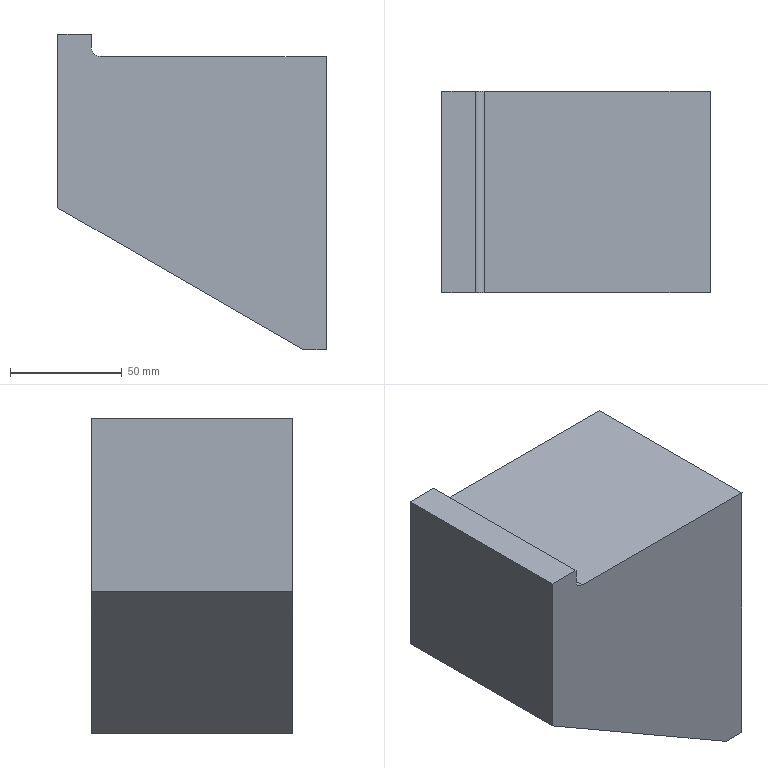Part | NX | features solid 2 | 1 solid | 10 faces | box 120 x 90 x 141.188 mm | volume 1116272 mm3 | plane 8 | spline 1 | cylinder 1 | commonest cylinder face diameters 8 x1
STEP:
#1=CARTESIAN_POINT('',(-871.,-430.,-90.));
#2=VERTEX_POINT('',#1);
#3=CARTESIAN_POINT('',(-770.,-430.,-90.));
#4=VERTEX_POINT('',#3);
#5=CARTESIAN_POINT('',(-871.,-430.,-90.));
#6=CARTESIAN_POINT('',(-837.333,-430.,-90.));
#7=CARTESIAN_POINT('',(-803.667,-430.,-90.));
#8=CARTESIAN_POINT('',(-770.,-430.,-90.));
#9=B_SPLINE_CURVE_WITH_KNOTS('',3,(#5,#6,#7,#8),.UNSPECIFIED.,.F.,.F.,(4,4),(0.1583,1.),.UNSPECIFIED.);
#10=EDGE_CURVE('',#2,#4,#9,.T.);
#11=ORIENTED_EDGE('',*,*,#10,.T.);
#12=CARTESIAN_POINT('',(-770.,-340.,-90.));
#13=VERTEX_POINT('',#12);
#14=CARTESIAN_POINT('',(-770.,-430.,-90.));
#15=CARTESIAN_POINT('',(-770.,-400.,-90.));
#16=CARTESIAN_POINT('',(-770.,-370.,-90.));
#17=CARTESIAN_POINT('',(-770.,-340.,-90.));
#18=B_SPLINE_CURVE_WITH_KNOTS('',3,(#14,#15,#16,#17),.UNSPECIFIED.,.F.,.F.,(4,4),(0.,1.),.UNSPECIFIED.);
#19=EDGE_CURVE('',#4,#13,#18,.T.);
#20=ORIENTED_EDGE('',*,*,#19,.T.);
#21=CARTESIAN_POINT('',(-871.,-340.,-90.));
#22=VERTEX_POINT('',#21);
#23=CARTESIAN_POINT('',(-770.,-340.,-90.));
#24=CARTESIAN_POINT('',(-803.667,-340.,-90.));
#25=CARTESIAN_POINT('',(-837.333,-340.,-90.));
#26=CARTESIAN_POINT('',(-871.,-340.,-90.));
#27=B_SPLINE_CURVE_WITH_KNOTS('',3,(#23,#24,#25,#26),.UNSPECIFIED.,.F.,.F.,(4,4),(0.,0.8417),.UNSPECIFIED.);
#28=EDGE_CURVE('',#22,#13,#27,.F.);
#29=ORIENTED_EDGE('',*,*,#28,.F.);
#30=CARTESIAN_POINT('',(-871.,-385.,-90.));
#31=DIRECTION('',(0.000000011,1.,0.00000017));
#32=VECTOR('',#31,1000.);
#33=LINE('',#30,#32);
#34=EDGE_CURVE('',#2,#22,#33,.T.);
#35=ORIENTED_EDGE('',*,*,#34,.F.);
#36=EDGE_LOOP('',(#11,#20,#29,#35));
#37=FACE_BOUND('',#36,.T.);
#38=CARTESIAN_POINT('',(-890.,-385.,-90.));
#39=DIRECTION('',(0.000000341,-0.00000017,1.));
#40=DIRECTION('',(-1.,0.000000011,0.000000341));
#41=AXIS2_PLACEMENT_3D('',#38,#39,#40);
#42=PLANE('',#41);
#43=ADVANCED_FACE('',(#37),#42,.T.);
#44=CARTESIAN_POINT('',(-780.,-430.,-221.188));
#45=VERTEX_POINT('',#44);
#46=CARTESIAN_POINT('',(-770.,-430.,-221.188));
#47=VERTEX_POINT('',#46);
#48=CARTESIAN_POINT('',(-780.,-430.,-221.188));
#49=CARTESIAN_POINT('',(-776.667,-430.,-221.188));
#50=CARTESIAN_POINT('',(-773.333,-430.,-221.188));
#51=CARTESIAN_POINT('',(-770.,-430.,-221.188));
#52=B_SPLINE_CURVE_WITH_KNOTS('',3,(#48,#49,#50,#51),.UNSPECIFIED.,.F.,.F.,(4,4),(0.9167,1.),.UNSPECIFIED.);
#53=EDGE_CURVE('',#45,#47,#52,.T.);
#54=ORIENTED_EDGE('',*,*,#53,.T.);
#55=CARTESIAN_POINT('',(-770.,-430.,-221.188));
#56=CARTESIAN_POINT('',(-770.,-430.,-177.458));
#57=CARTESIAN_POINT('',(-770.,-430.,-133.729));
#58=CARTESIAN_POINT('',(-770.,-430.,-90.));
#59=B_SPLINE_CURVE_WITH_KNOTS('',3,(#55,#56,#57,#58),.UNSPECIFIED.,.F.,.F.,(4,4),(0.,1.),.UNSPECIFIED.);
#60=EDGE_CURVE('',#47,#4,#59,.T.);
#61=ORIENTED_EDGE('',*,*,#60,.T.);
#62=ORIENTED_EDGE('',*,*,#10,.F.);
#63=CARTESIAN_POINT('',(-875.,-430.,-86.));
#64=VERTEX_POINT('',#63);
#65=CARTESIAN_POINT('',(-871.,-430.,-86.));
#66=DIRECTION('',(0.000000011,1.,0.00000017));
#67=DIRECTION('',(-0.000000341,0.00000017,-1.));
#68=AXIS2_PLACEMENT_3D('',#65,#66,#67);
#69=CIRCLE('',#68,4.);
#70=EDGE_CURVE('',#64,#2,#69,.F.);
#71=ORIENTED_EDGE('',*,*,#70,.F.);
#72=CARTESIAN_POINT('',(-875.,-430.,-80.));
#73=VERTEX_POINT('',#72);
#74=CARTESIAN_POINT('',(-875.,-430.,-90.));
#75=DIRECTION('',(-0.000000341,0.00000017,-1.));
#76=VECTOR('',#75,1000.);
#77=LINE('',#74,#76);
#78=EDGE_CURVE('',#64,#73,#77,.F.);
#79=ORIENTED_EDGE('',*,*,#78,.T.);
#80=CARTESIAN_POINT('',(-890.,-430.,-80.));
#81=VERTEX_POINT('',#80);
#82=CARTESIAN_POINT('',(-890.,-430.,-80.));
#83=DIRECTION('',(-1.,0.000000011,0.000000341));
#84=VECTOR('',#83,1000.);
#85=LINE('',#82,#84);
#86=EDGE_CURVE('',#73,#81,#85,.T.);
#87=ORIENTED_EDGE('',*,*,#86,.T.);
#88=CARTESIAN_POINT('',(-890.,-430.,-90.));
#89=VERTEX_POINT('',#88);
#90=CARTESIAN_POINT('',(-890.,-430.,-90.));
#91=DIRECTION('',(0.000000341,-0.00000017,1.));
#92=VECTOR('',#91,1000.);
#93=LINE('',#90,#92);
#94=EDGE_CURVE('',#89,#81,#93,.T.);
#95=ORIENTED_EDGE('',*,*,#94,.F.);
#96=CARTESIAN_POINT('',(-890.,-430.,-157.679));
#97=VERTEX_POINT('',#96);
#98=CARTESIAN_POINT('',(-890.,-430.,-90.));
#99=CARTESIAN_POINT('',(-890.,-430.,-112.56));
#100=CARTESIAN_POINT('',(-890.,-430.,-135.119));
#101=CARTESIAN_POINT('',(-890.,-430.,-157.679));
#102=B_SPLINE_CURVE_WITH_KNOTS('',3,(#98,#99,#100,#101),.UNSPECIFIED.,.F.,.F.,(4,4),(0.,0.5159),.UNSPECIFIED.);
#103=EDGE_CURVE('',#97,#89,#102,.F.);
#104=ORIENTED_EDGE('',*,*,#103,.F.);
#105=CARTESIAN_POINT('',(-890.903,-430.,-157.158));
#106=DIRECTION('',(-0.866,-0.000000076,0.5));
#107=VECTOR('',#106,1000.);
#108=LINE('',#105,#107);
#109=EDGE_CURVE('',#45,#97,#108,.T.);
#110=ORIENTED_EDGE('',*,*,#109,.F.);
#111=EDGE_LOOP('',(#54,#61,#62,#71,#79,#87,#95,#104,#110));
#112=FACE_BOUND('',#111,.T.);
#113=CARTESIAN_POINT('',(-890.,-430.,-155.594));
#114=DIRECTION('',(-0.000000011,-1.,-0.00000017));
#115=DIRECTION('',(-0.000000341,0.00000017,-1.));
#116=AXIS2_PLACEMENT_3D('',#113,#114,#115);
#117=PLANE('',#116);
#118=ADVANCED_FACE('',(#112),#117,.T.);
#119=CARTESIAN_POINT('',(-890.,-340.,-157.679));
#120=VERTEX_POINT('',#119);
#121=CARTESIAN_POINT('',(-890.,-340.,-90.));
#122=VERTEX_POINT('',#121);
#123=CARTESIAN_POINT('',(-890.,-340.,-157.679));
#124=CARTESIAN_POINT('',(-890.,-340.,-135.119));
#125=CARTESIAN_POINT('',(-890.,-340.,-112.56));
#126=CARTESIAN_POINT('',(-890.,-340.,-90.));
#127=B_SPLINE_CURVE_WITH_KNOTS('',3,(#123,#124,#125,#126),.UNSPECIFIED.,.F.,.F.,(4,4),(0.4841,1.),.UNSPECIFIED.);
#128=EDGE_CURVE('',#120,#122,#127,.T.);
#129=ORIENTED_EDGE('',*,*,#128,.T.);
#130=CARTESIAN_POINT('',(-890.,-340.,-80.));
#131=VERTEX_POINT('',#130);
#132=CARTESIAN_POINT('',(-890.,-340.,-90.));
#133=DIRECTION('',(0.000000341,-0.00000017,1.));
#134=VECTOR('',#133,1000.);
#135=LINE('',#132,#134);
#136=EDGE_CURVE('',#122,#131,#135,.T.);
#137=ORIENTED_EDGE('',*,*,#136,.T.);
#138=CARTESIAN_POINT('',(-875.,-340.,-80.));
#139=VERTEX_POINT('',#138);
#140=CARTESIAN_POINT('',(-890.,-340.,-80.));
#141=DIRECTION('',(-1.,0.000000011,0.000000341));
#142=VECTOR('',#141,1000.);
#143=LINE('',#140,#142);
#144=EDGE_CURVE('',#139,#131,#143,.T.);
#145=ORIENTED_EDGE('',*,*,#144,.F.);
#146=CARTESIAN_POINT('',(-875.,-340.,-86.));
#147=VERTEX_POINT('',#146);
#148=CARTESIAN_POINT('',(-875.,-340.,-90.));
#149=DIRECTION('',(-0.000000341,0.00000017,-1.));
#150=VECTOR('',#149,1000.);
#151=LINE('',#148,#150);
#152=EDGE_CURVE('',#147,#139,#151,.F.);
#153=ORIENTED_EDGE('',*,*,#152,.F.);
#154=CARTESIAN_POINT('',(-871.,-340.,-86.));
#155=DIRECTION('',(-0.000000011,-1.,-0.00000017));
#156=DIRECTION('',(0.000000341,-0.00000017,1.));
#157=AXIS2_PLACEMENT_3D('',#154,#155,#156);
#158=CIRCLE('',#157,4.);
#159=EDGE_CURVE('',#22,#147,#158,.F.);
#160=ORIENTED_EDGE('',*,*,#159,.F.);
#161=ORIENTED_EDGE('',*,*,#28,.T.);
#162=CARTESIAN_POINT('',(-770.,-340.,-221.188));
#163=VERTEX_POINT('',#162);
#164=CARTESIAN_POINT('',(-770.,-340.,-90.));
#165=CARTESIAN_POINT('',(-770.,-340.,-133.729));
#166=CARTESIAN_POINT('',(-770.,-340.,-177.458));
#167=CARTESIAN_POINT('',(-770.,-340.,-221.188));
#168=B_SPLINE_CURVE_WITH_KNOTS('',3,(#164,#165,#166,#167),.UNSPECIFIED.,.F.,.F.,(4,4),(0.,1.),.UNSPECIFIED.);
#169=EDGE_CURVE('',#13,#163,#168,.T.);
#170=ORIENTED_EDGE('',*,*,#169,.T.);
#171=CARTESIAN_POINT('',(-780.,-340.,-221.188));
#172=VERTEX_POINT('',#171);
#173=CARTESIAN_POINT('',(-770.,-340.,-221.188));
#174=CARTESIAN_POINT('',(-773.333,-340.,-221.188));
#175=CARTESIAN_POINT('',(-776.667,-340.,-221.188));
#176=CARTESIAN_POINT('',(-780.,-340.,-221.188));
#177=B_SPLINE_CURVE_WITH_KNOTS('',3,(#173,#174,#175,#176),.UNSPECIFIED.,.F.,.F.,(4,4),(0.,0.08333),.UNSPECIFIED.);
#178=EDGE_CURVE('',#172,#163,#177,.F.);
#179=ORIENTED_EDGE('',*,*,#178,.F.);
#180=CARTESIAN_POINT('',(-890.903,-340.,-157.158));
#181=DIRECTION('',(0.866,0.000000076,-0.5));
#182=VECTOR('',#181,1000.);
#183=LINE('',#180,#182);
#184=EDGE_CURVE('',#120,#172,#183,.T.);
#185=ORIENTED_EDGE('',*,*,#184,.F.);
#186=EDGE_LOOP('',(#129,#137,#145,#153,#160,#161,#170,#179,#185));
#187=FACE_BOUND('',#186,.T.);
#188=CARTESIAN_POINT('',(-890.,-340.,-155.594));
#189=DIRECTION('',(0.000000011,1.,0.00000017));
#190=DIRECTION('',(0.000000341,-0.00000017,1.));
#191=AXIS2_PLACEMENT_3D('',#188,#189,#190);
#192=PLANE('',#191);
#193=ADVANCED_FACE('',(#187),#192,.T.);
#194=ORIENTED_EDGE('',*,*,#178,.T.);
#195=CARTESIAN_POINT('',(-770.,-340.,-221.188));
#196=CARTESIAN_POINT('',(-770.,-370.,-221.188));
#197=CARTESIAN_POINT('',(-770.,-400.,-221.188));
#198=CARTESIAN_POINT('',(-770.,-430.,-221.188));
#199=B_SPLINE_CURVE_WITH_KNOTS('',3,(#195,#196,#197,#198),.UNSPECIFIED.,.F.,.F.,(4,4),(0.,1.),.UNSPECIFIED.);
#200=EDGE_CURVE('',#163,#47,#199,.T.);
#201=ORIENTED_EDGE('',*,*,#200,.T.);
#202=ORIENTED_EDGE('',*,*,#53,.F.);
#203=CARTESIAN_POINT('',(-780.,-430.,-221.188));
#204=DIRECTION('',(-0.000000011,-1.,-0.00000017));
#205=VECTOR('',#204,1000.);
#206=LINE('',#203,#205);
#207=EDGE_CURVE('',#172,#45,#206,.T.);
#208=ORIENTED_EDGE('',*,*,#207,.F.);
#209=EDGE_LOOP('',(#194,#201,#202,#208));
#210=FACE_BOUND('',#209,.T.);
#211=CARTESIAN_POINT('',(-890.,-385.,-221.188));
#212=DIRECTION('',(-0.000000341,0.00000017,-1.));
#213=DIRECTION('',(1.,-0.000000011,-0.000000341));
#214=AXIS2_PLACEMENT_3D('',#211,#212,#213);
#215=PLANE('',#214);
#216=ADVANCED_FACE('',(#210),#215,.T.);
#217=ORIENTED_EDGE('',*,*,#103,.T.);
#218=ORIENTED_EDGE('',*,*,#94,.T.);
#219=CARTESIAN_POINT('',(-890.,-430.,-80.));
#220=CARTESIAN_POINT('',(-890.,-340.,-80.));
#221=B_SPLINE_CURVE_WITH_KNOTS('',1,(#219,#220),.UNSPECIFIED.,.F.,.F.,(2,2),(0.,1.),.PIECEWISE_BEZIER_KNOTS.);
#222=EDGE_CURVE('',#81,#131,#221,.T.);
#223=ORIENTED_EDGE('',*,*,#222,.T.);
#224=ORIENTED_EDGE('',*,*,#136,.F.);
#225=ORIENTED_EDGE('',*,*,#128,.F.);
#226=CARTESIAN_POINT('',(-890.,-340.,-157.679));
#227=DIRECTION('',(0.000000011,1.,0.00000017));
#228=VECTOR('',#227,1000.);
#229=LINE('',#226,#228);
#230=EDGE_CURVE('',#97,#120,#229,.T.);
#231=ORIENTED_EDGE('',*,*,#230,.F.);
#232=EDGE_LOOP('',(#217,#218,#223,#224,#225,#231));
#233=FACE_BOUND('',#232,.T.);
#234=CARTESIAN_POINT('',(-890.,-385.,-155.594));
#235=DIRECTION('',(1.,-0.000000011,-0.000000341));
#236=DIRECTION('',(-0.000000011,-1.,-0.00000017));
#237=AXIS2_PLACEMENT_3D('',#234,#235,#236);
#238=PLANE('',#237);
#239=ADVANCED_FACE('',(#233),#238,.F.);
#240=ORIENTED_EDGE('',*,*,#60,.F.);
#241=ORIENTED_EDGE('',*,*,#200,.F.);
#242=ORIENTED_EDGE('',*,*,#169,.F.);
#243=ORIENTED_EDGE('',*,*,#19,.F.);
#244=EDGE_LOOP('',(#240,#241,#242,#243));
#245=FACE_BOUND('',#244,.T.);
#246=CARTESIAN_POINT('',(-770.,-385.,-155.594));
#247=DIRECTION('',(1.,-0.000000011,-0.000000341));
#248=DIRECTION('',(-0.000000011,-1.,-0.00000017));
#249=AXIS2_PLACEMENT_3D('',#246,#247,#248);
#250=PLANE('',#249);
#251=ADVANCED_FACE('',(#245),#250,.T.);
#252=ORIENTED_EDGE('',*,*,#184,.T.);
#253=ORIENTED_EDGE('',*,*,#207,.T.);
#254=ORIENTED_EDGE('',*,*,#109,.T.);
#255=ORIENTED_EDGE('',*,*,#230,.T.);
#256=EDGE_LOOP('',(#252,#253,#254,#255));
#257=FACE_BOUND('',#256,.T.);
#258=CARTESIAN_POINT('',(-780.,-385.,-221.188));
#259=DIRECTION('',(-0.5,0.000000153,-0.866));
#260=DIRECTION('',(0.866,0.000000076,-0.5));
#261=AXIS2_PLACEMENT_3D('',#258,#259,#260);
#262=PLANE('',#261);
#263=ADVANCED_FACE('',(#257),#262,.T.);
#264=ORIENTED_EDGE('',*,*,#144,.T.);
#265=ORIENTED_EDGE('',*,*,#222,.F.);
#266=ORIENTED_EDGE('',*,*,#86,.F.);
#267=CARTESIAN_POINT('',(-875.,-430.,-80.));
#268=CARTESIAN_POINT('',(-875.,-340.,-80.));
#269=B_SPLINE_CURVE_WITH_KNOTS('',1,(#267,#268),.UNSPECIFIED.,.F.,.F.,(2,2),(0.,1.),.UNSPECIFIED.);
#270=EDGE_CURVE('',#73,#139,#269,.T.);
#271=ORIENTED_EDGE('',*,*,#270,.T.);
#272=EDGE_LOOP('',(#264,#265,#266,#271));
#273=FACE_BOUND('',#272,.T.);
#274=CARTESIAN_POINT('',(-875.,-430.,-80.));
#275=CARTESIAN_POINT('',(-890.,-430.,-80.));
#276=CARTESIAN_POINT('',(-875.,-340.,-80.));
#277=CARTESIAN_POINT('',(-890.,-340.,-80.));
#278=B_SPLINE_SURFACE_WITH_KNOTS('',1,1,((#274,#275),(#276,#277)),.SURF_OF_LINEAR_EXTRUSION.,.F.,.F.,.F.,(2,2),(2,2),(0.,1.),(0.,1.),.PIECEWISE_BEZIER_KNOTS.);
#279=ADVANCED_FACE('',(#273),#278,.T.);
#280=ORIENTED_EDGE('',*,*,#152,.T.);
#281=ORIENTED_EDGE('',*,*,#270,.F.);
#282=ORIENTED_EDGE('',*,*,#78,.F.);
#283=CARTESIAN_POINT('',(-875.,-430.,-86.));
#284=DIRECTION('',(0.000000011,1.,0.00000017));
#285=VECTOR('',#284,1000.);
#286=LINE('',#283,#285);
#287=EDGE_CURVE('',#147,#64,#286,.F.);
#288=ORIENTED_EDGE('',*,*,#287,.F.);
#289=EDGE_LOOP('',(#280,#281,#282,#288));
#290=FACE_BOUND('',#289,.T.);
#291=CARTESIAN_POINT('',(-875.,-430.,-90.));
#292=DIRECTION('',(-1.,0.000000011,0.000000341));
#293=DIRECTION('',(-0.000000341,0.00000017,-1.));
#294=AXIS2_PLACEMENT_3D('',#291,#292,#293);
#295=PLANE('',#294);
#296=ADVANCED_FACE('',(#290),#295,.F.);
#297=ORIENTED_EDGE('',*,*,#70,.T.);
#298=ORIENTED_EDGE('',*,*,#34,.T.);
#299=ORIENTED_EDGE('',*,*,#159,.T.);
#300=ORIENTED_EDGE('',*,*,#287,.T.);
#301=EDGE_LOOP('',(#297,#298,#299,#300));
#302=FACE_BOUND('',#301,.T.);
#303=CARTESIAN_POINT('',(-871.,-385.,-86.));
#304=DIRECTION('',(0.000000011,1.,0.00000017));
#305=DIRECTION('',(0.000000341,-0.00000017,1.));
#306=AXIS2_PLACEMENT_3D('',#303,#304,#305);
#307=CYLINDRICAL_SURFACE('',#306,4.);
#308=ADVANCED_FACE('',(#302),#307,.F.);
#309=CLOSED_SHELL('',(#43,#118,#193,#216,#239,#251,#263,#279,#296,#308));
#310=MANIFOLD_SOLID_BREP('',#309);
#311=(LENGTH_UNIT()NAMED_UNIT(*)SI_UNIT(.MILLI.,.METRE.));
#312=UNCERTAINTY_MEASURE_WITH_UNIT(LENGTH_MEASURE(0.0508),#311,'','');
#313=(NAMED_UNIT(*)PLANE_ANGLE_UNIT()SI_UNIT($,.RADIAN.));
#314=(NAMED_UNIT(*)SI_UNIT($,.STERADIAN.)SOLID_ANGLE_UNIT());
#315=(GEOMETRIC_REPRESENTATION_CONTEXT(3)GLOBAL_UNCERTAINTY_ASSIGNED_CONTEXT((#312))GLOBAL_UNIT_ASSIGNED_CONTEXT((#311,#313,#314))REPRESENTATION_CONTEXT('',''));
#316=ADVANCED_BREP_SHAPE_REPRESENTATION('',(#310),#315);